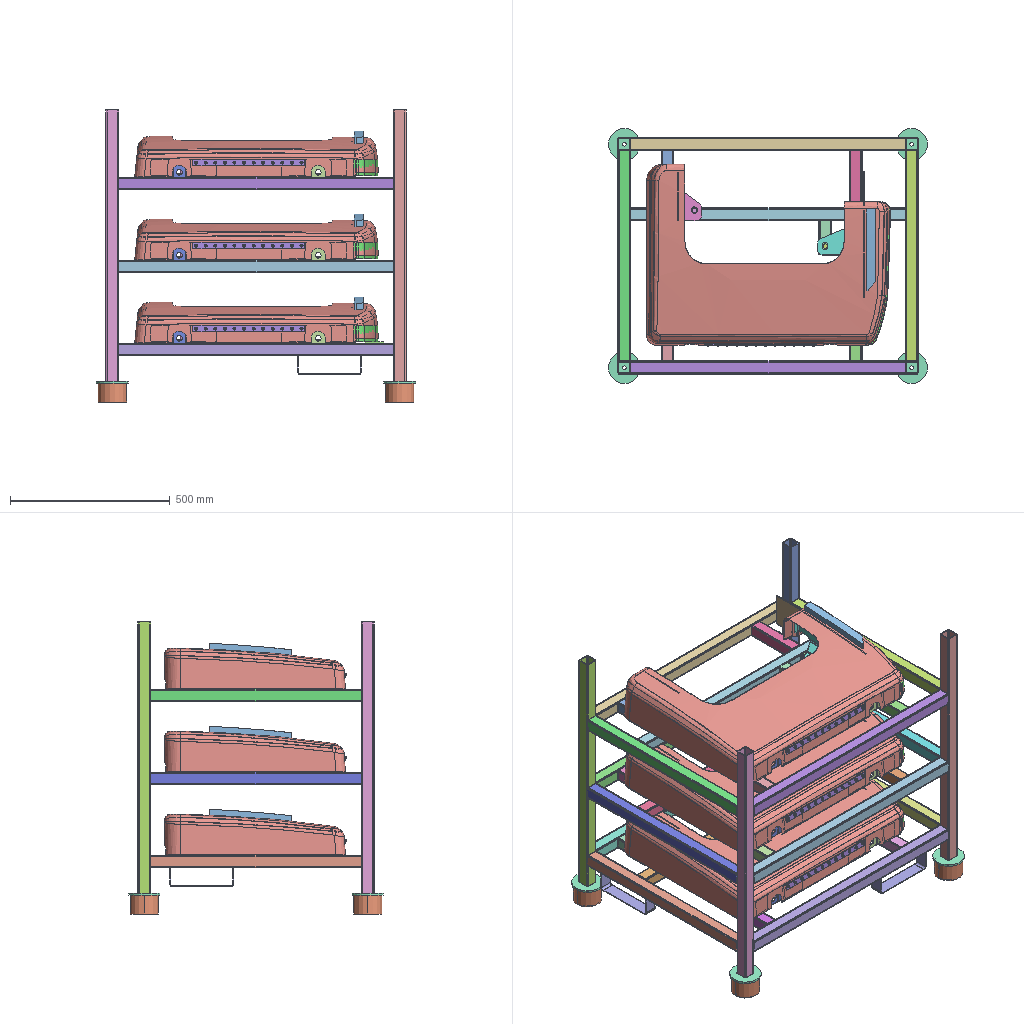Assembly | SolidWorks | 7 different items | 22 placed | box 1000 x 798 x 915 mm
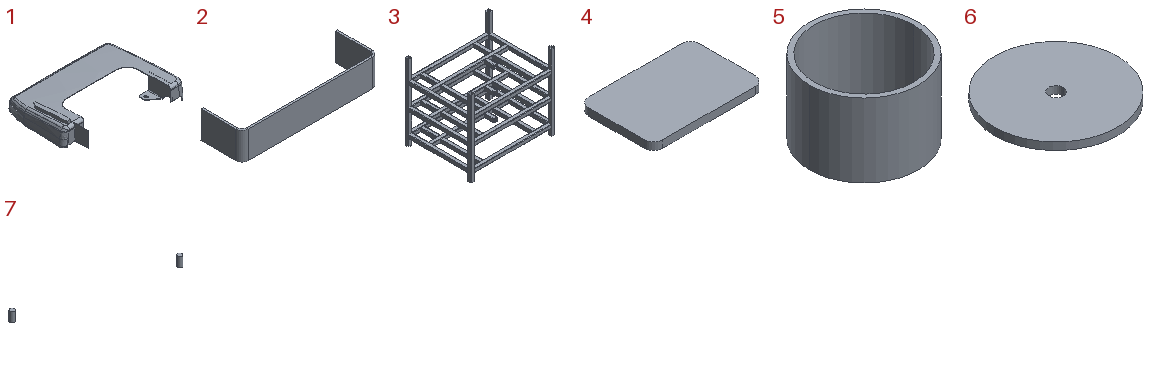Parts list (item | quantity | size | volume | features):
1 | x3 | 763.446 x 569.652 x 148.304 mm | 1530854 mm3 | features BaseBody 10
2 | x4 | 200 x 60 x 40 mm | 36907 mm3 | features FlatPattern 1, SMBaseFlange 1, SheetMetal 1
3 | x1 | 940 x 740 x 850 mm | 8249556 mm3 | features 3DProfileFeature 1, WeldMemberFeat 1, WeldmentFeature 1
4 | x3 | 60 x 40 x 4 mm | 9514 mm3 | features FlatPattern 1, SMBaseFlange 1, SheetMetal 1
5 | x4 | 89 x 89 x 60 mm | 64088 mm3 | features Extrusion 1
6 | x4 | 100 x 100 x 6 mm | 46445 mm3 | features FlatPattern 1, SMBaseFlange 1, SheetMetal 1
7 | x3 | 423.435 x 126.4 x 30 mm | 9236 mm3 | features Extrusion 1
Mates (type | each side: item.copy, entity, surface, feature):
Coincident | 3.1 face plane GB/6728-1986 square hollow section 40 X 40 X 3(1) | 1.1 face plane 2A3-54-17270_ASM.stp-1/2A3-54-17A10_ASM.stp-1/2A3-54-17A10-01.stp-1-solid1
DistanceDim | 3.1 face plane GB/6728-1986 square hollow section 40 X 40 X 3(1) | 1.1 edge
DistanceDim | 1.1 edge | 3.1 face plane GB/6728-1986 square hollow section 40 X 40 X 3(1)
InPlace | 3.1 face plane GB/6728-1986 square hollow section 40 X 40 X 3(1) | 7.1 plane
Coincident | 3.1 face plane GB/6728-1986 square hollow section 40 X 40 X 3(1) | 6.1 face plane Base-Flange1
DistanceDim | 6.1 face cylinder Base-Flange1 | 3.1 face plane GB/6728-1986 square hollow section 40 X 40 X 3(1)
DistanceDim | 3.1 face plane GB/6728-1986 square hollow section 40 X 40 X 3(1) | 6.1 face cylinder Base-Flange1
Concentric | 6.1 face cylinder Base-Flange1 | 5.1 face cylinder Boss-Extrude1
Coincident | 3.1 face plane GB/6728-1986 square hollow section 40 X 40 X 3(1) | 2.1 face plane Base-Flange1 | 2 times
DistanceDim | 2.1 face plane Base-Flange1 | 3.1 face plane GB/6728-1986 square hollow section 40 X 40 X 3(1)
Coincident | 3.1 face plane GB/6728-1986 square hollow section 40 X 40 X 3(1) | 2.2 face plane Base-Flange1 | 2 times
DistanceDim | 2.2 face plane Base-Flange1 | 3.1 face plane GB/6728-1986 square hollow section 40 X 40 X 3(1)
Coincident | 3.1 face plane GB/6728-1986 square hollow section 40 X 40 X 3(1) | 4.1 face plane Base-Flange1 | 2 times
DistanceDim | 4.1 face plane Base-Flange1 | 3.1 face plane GB/6728-1986 square hollow section 40 X 40 X 3(1)